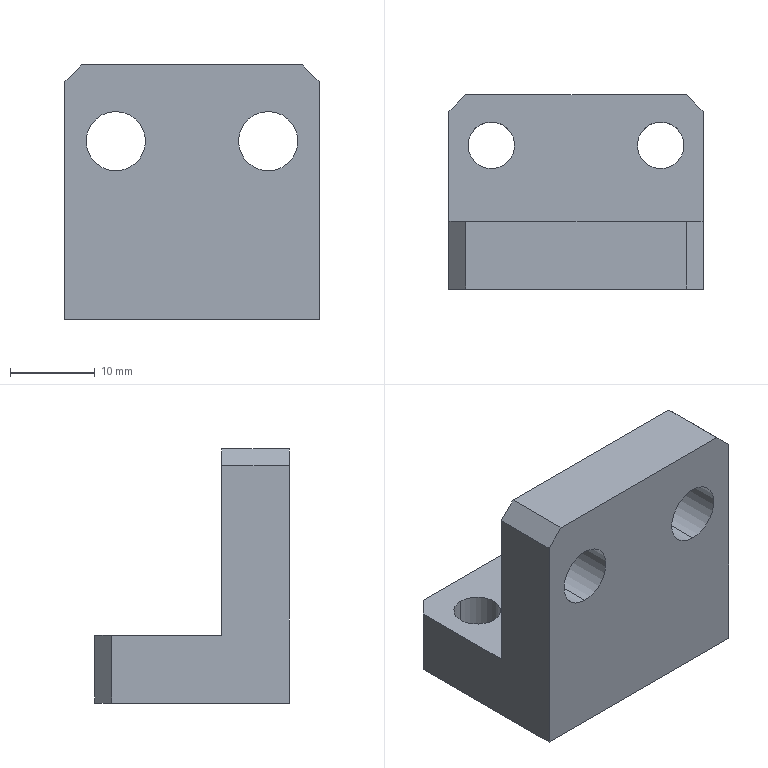Part | SolidWorks | features BaseBody 1 | 1 solid | 20 faces | box 30.001 x 23.001 x 30 mm | volume 9740 mm3 | plane 12 | cylinder 8 | commonest cylinder face diameters 5.5 x4 7 x4
STEP:
#1=CARTESIAN_POINT('',(-621.131,675.797,346.732));
#2=VERTEX_POINT('',#1);
#3=CARTESIAN_POINT('',(-619.131,675.797,344.732));
#4=VERTEX_POINT('',#3);
#5=CARTESIAN_POINT('',(-621.131,675.797,346.732));
#6=DIRECTION('',(0.7071,-0.00003242,-0.7071));
#7=VECTOR('',#6,1000.);
#8=LINE('',#5,#7);
#9=EDGE_CURVE('',#2,#4,#8,.T.);
#10=ORIENTED_EDGE('',*,*,#9,.T.);
#11=CARTESIAN_POINT('',(-619.131,683.797,344.732));
#12=VERTEX_POINT('',#11);
#13=CARTESIAN_POINT('',(-619.131,683.797,344.732));
#14=DIRECTION('',(-0.00004584,-1.,0.));
#15=VECTOR('',#14,1000.);
#16=LINE('',#13,#15);
#17=EDGE_CURVE('',#12,#4,#16,.T.);
#18=ORIENTED_EDGE('',*,*,#17,.F.);
#19=CARTESIAN_POINT('',(-621.131,683.797,346.732));
#20=VERTEX_POINT('',#19);
#21=CARTESIAN_POINT('',(-619.131,683.797,344.732));
#22=DIRECTION('',(-0.7071,0.00003242,0.7071));
#23=VECTOR('',#22,1000.);
#24=LINE('',#21,#23);
#25=EDGE_CURVE('',#12,#20,#24,.T.);
#26=ORIENTED_EDGE('',*,*,#25,.T.);
#27=CARTESIAN_POINT('',(-621.131,675.797,346.732));
#28=DIRECTION('',(0.00004584,1.,0.));
#29=VECTOR('',#28,1000.);
#30=LINE('',#27,#29);
#31=EDGE_CURVE('',#2,#20,#30,.T.);
#32=ORIENTED_EDGE('',*,*,#31,.F.);
#33=EDGE_LOOP('',(#10,#18,#26,#32));
#34=FACE_OUTER_BOUND('',#33,.T.);
#35=CARTESIAN_POINT('',(-619.131,675.797,344.732));
#36=DIRECTION('',(-0.7071,0.00003242,-0.7071));
#37=DIRECTION('',(0.00004584,1.,0.));
#38=AXIS2_PLACEMENT_3D('',#35,#36,#37);
#39=PLANE('',#38);
#40=ADVANCED_FACE('',(#34),#39,.F.);
#41=CARTESIAN_POINT('',(-647.131,675.798,346.732));
#42=VERTEX_POINT('',#41);
#43=CARTESIAN_POINT('',(-647.131,675.798,346.732));
#44=DIRECTION('',(1.,-0.00004584,0.));
#45=VECTOR('',#44,1000.);
#46=LINE('',#43,#45);
#47=EDGE_CURVE('',#42,#2,#46,.T.);
#48=ORIENTED_EDGE('',*,*,#47,.T.);
#49=ORIENTED_EDGE('',*,*,#31,.T.);
#50=CARTESIAN_POINT('',(-647.131,683.798,346.732));
#51=VERTEX_POINT('',#50);
#52=CARTESIAN_POINT('',(-621.131,683.797,346.732));
#53=DIRECTION('',(-1.,0.00004584,0.));
#54=VECTOR('',#53,1000.);
#55=LINE('',#52,#54);
#56=EDGE_CURVE('',#20,#51,#55,.T.);
#57=ORIENTED_EDGE('',*,*,#56,.T.);
#58=CARTESIAN_POINT('',(-647.131,675.798,346.732));
#59=DIRECTION('',(0.00004584,1.,0.));
#60=VECTOR('',#59,1000.);
#61=LINE('',#58,#60);
#62=EDGE_CURVE('',#42,#51,#61,.T.);
#63=ORIENTED_EDGE('',*,*,#62,.F.);
#64=EDGE_LOOP('',(#48,#49,#57,#63));
#65=FACE_OUTER_BOUND('',#64,.T.);
#66=CARTESIAN_POINT('',(-619.131,675.797,346.732));
#67=DIRECTION('',(0.,0.,-1.));
#68=DIRECTION('',(-0.00004584,-1.,0.));
#69=AXIS2_PLACEMENT_3D('',#66,#67,#68);
#70=PLANE('',#69);
#71=ADVANCED_FACE('',(#65),#70,.F.);
#72=CARTESIAN_POINT('',(-649.131,675.798,344.732));
#73=VERTEX_POINT('',#72);
#74=CARTESIAN_POINT('',(-649.131,675.798,344.732));
#75=DIRECTION('',(0.7071,-0.00003242,0.7071));
#76=VECTOR('',#75,1000.);
#77=LINE('',#74,#76);
#78=EDGE_CURVE('',#73,#42,#77,.T.);
#79=ORIENTED_EDGE('',*,*,#78,.T.);
#80=ORIENTED_EDGE('',*,*,#62,.T.);
#81=CARTESIAN_POINT('',(-649.131,683.798,344.732));
#82=VERTEX_POINT('',#81);
#83=CARTESIAN_POINT('',(-647.131,683.798,346.732));
#84=DIRECTION('',(-0.7071,0.00003242,-0.7071));
#85=VECTOR('',#84,1000.);
#86=LINE('',#83,#85);
#87=EDGE_CURVE('',#51,#82,#86,.T.);
#88=ORIENTED_EDGE('',*,*,#87,.T.);
#89=CARTESIAN_POINT('',(-649.131,683.798,344.732));
#90=DIRECTION('',(-0.00004584,-1.,0.));
#91=VECTOR('',#90,1000.);
#92=LINE('',#89,#91);
#93=EDGE_CURVE('',#82,#73,#92,.T.);
#94=ORIENTED_EDGE('',*,*,#93,.T.);
#95=EDGE_LOOP('',(#79,#80,#88,#94));
#96=FACE_OUTER_BOUND('',#95,.T.);
#97=CARTESIAN_POINT('',(-647.131,675.798,346.732));
#98=DIRECTION('',(-0.7071,0.00003242,0.7071));
#99=DIRECTION('',(-0.00004584,-1.,0.));
#100=AXIS2_PLACEMENT_3D('',#97,#98,#99);
#101=PLANE('',#100);
#102=ADVANCED_FACE('',(#96),#101,.T.);
#103=CARTESIAN_POINT('',(-649.131,675.798,316.732));
#104=VERTEX_POINT('',#103);
#105=CARTESIAN_POINT('',(-649.13,696.798,316.732));
#106=VERTEX_POINT('',#105);
#107=CARTESIAN_POINT('',(-649.131,675.798,316.732));
#108=DIRECTION('',(0.00004584,1.,0.));
#109=VECTOR('',#108,1000.);
#110=LINE('',#107,#109);
#111=EDGE_CURVE('',#104,#106,#110,.T.);
#112=ORIENTED_EDGE('',*,*,#111,.F.);
#113=CARTESIAN_POINT('',(-649.131,675.798,344.732));
#114=DIRECTION('',(0.,0.,-1.));
#115=VECTOR('',#114,1000.);
#116=LINE('',#113,#115);
#117=EDGE_CURVE('',#73,#104,#116,.T.);
#118=ORIENTED_EDGE('',*,*,#117,.F.);
#119=ORIENTED_EDGE('',*,*,#93,.F.);
#120=CARTESIAN_POINT('',(-649.131,683.798,324.732));
#121=VERTEX_POINT('',#120);
#122=CARTESIAN_POINT('',(-649.131,683.798,344.732));
#123=DIRECTION('',(0.,0.,-1.));
#124=VECTOR('',#123,1000.);
#125=LINE('',#122,#124);
#126=EDGE_CURVE('',#82,#121,#125,.T.);
#127=ORIENTED_EDGE('',*,*,#126,.T.);
#128=CARTESIAN_POINT('',(-649.13,696.798,324.732));
#129=VERTEX_POINT('',#128);
#130=CARTESIAN_POINT('',(-649.13,696.798,324.732));
#131=DIRECTION('',(-0.00004584,-1.,0.));
#132=VECTOR('',#131,1000.);
#133=LINE('',#130,#132);
#134=EDGE_CURVE('',#129,#121,#133,.T.);
#135=ORIENTED_EDGE('',*,*,#134,.F.);
#136=CARTESIAN_POINT('',(-649.13,696.798,316.732));
#137=DIRECTION('',(0.,0.,1.));
#138=VECTOR('',#137,1000.);
#139=LINE('',#136,#138);
#140=EDGE_CURVE('',#106,#129,#139,.T.);
#141=ORIENTED_EDGE('',*,*,#140,.F.);
#142=EDGE_LOOP('',(#112,#118,#119,#127,#135,#141));
#143=FACE_OUTER_BOUND('',#142,.T.);
#144=CARTESIAN_POINT('',(-649.131,675.798,316.732));
#145=DIRECTION('',(-1.,0.00004584,0.));
#146=DIRECTION('',(0.,0.,-1.));
#147=AXIS2_PLACEMENT_3D('',#144,#145,#146);
#148=PLANE('',#147);
#149=ADVANCED_FACE('',(#143),#148,.T.);
#150=CARTESIAN_POINT('',(-647.13,698.798,324.732));
#151=VERTEX_POINT('',#150);
#152=CARTESIAN_POINT('',(-649.13,696.798,324.732));
#153=DIRECTION('',(0.7071,0.7071,0.));
#154=VECTOR('',#153,1000.);
#155=LINE('',#152,#154);
#156=EDGE_CURVE('',#129,#151,#155,.T.);
#157=ORIENTED_EDGE('',*,*,#156,.T.);
#158=CARTESIAN_POINT('',(-647.13,698.798,316.732));
#159=VERTEX_POINT('',#158);
#160=CARTESIAN_POINT('',(-647.13,698.798,324.732));
#161=DIRECTION('',(0.,0.,-1.));
#162=VECTOR('',#161,1000.);
#163=LINE('',#160,#162);
#164=EDGE_CURVE('',#151,#159,#163,.T.);
#165=ORIENTED_EDGE('',*,*,#164,.T.);
#166=CARTESIAN_POINT('',(-647.13,698.798,316.732));
#167=DIRECTION('',(-0.7071,-0.7071,0.));
#168=VECTOR('',#167,1000.);
#169=LINE('',#166,#168);
#170=EDGE_CURVE('',#159,#106,#169,.T.);
#171=ORIENTED_EDGE('',*,*,#170,.T.);
#172=ORIENTED_EDGE('',*,*,#140,.T.);
#173=EDGE_LOOP('',(#157,#165,#171,#172));
#174=FACE_OUTER_BOUND('',#173,.T.);
#175=CARTESIAN_POINT('',(-647.13,698.798,324.732));
#176=DIRECTION('',(-0.7071,0.7071,0.));
#177=DIRECTION('',(-0.7071,-0.7071,0.));
#178=AXIS2_PLACEMENT_3D('',#175,#176,#177);
#179=PLANE('',#178);
#180=ADVANCED_FACE('',(#174),#179,.T.);
#181=CARTESIAN_POINT('',(-621.13,698.797,316.732));
#182=VERTEX_POINT('',#181);
#183=CARTESIAN_POINT('',(-647.13,698.798,316.732));
#184=DIRECTION('',(1.,-0.00004584,0.));
#185=VECTOR('',#184,1000.);
#186=LINE('',#183,#185);
#187=EDGE_CURVE('',#159,#182,#186,.T.);
#188=ORIENTED_EDGE('',*,*,#187,.T.);
#189=CARTESIAN_POINT('',(-619.13,696.797,316.732));
#190=VERTEX_POINT('',#189);
#191=CARTESIAN_POINT('',(-619.13,696.797,316.732));
#192=DIRECTION('',(-0.7071,0.7071,0.));
#193=VECTOR('',#192,1000.);
#194=LINE('',#191,#193);
#195=EDGE_CURVE('',#190,#182,#194,.T.);
#196=ORIENTED_EDGE('',*,*,#195,.F.);
#197=CARTESIAN_POINT('',(-619.131,675.797,316.732));
#198=VERTEX_POINT('',#197);
#199=CARTESIAN_POINT('',(-619.131,675.797,316.732));
#200=DIRECTION('',(0.00004584,1.,0.));
#201=VECTOR('',#200,1000.);
#202=LINE('',#199,#201);
#203=EDGE_CURVE('',#198,#190,#202,.T.);
#204=ORIENTED_EDGE('',*,*,#203,.F.);
#205=CARTESIAN_POINT('',(-649.131,675.798,316.732));
#206=DIRECTION('',(1.,-0.00004584,0.));
#207=VECTOR('',#206,1000.);
#208=LINE('',#205,#207);
#209=EDGE_CURVE('',#104,#198,#208,.T.);
#210=ORIENTED_EDGE('',*,*,#209,.F.);
#211=ORIENTED_EDGE('',*,*,#111,.T.);
#212=ORIENTED_EDGE('',*,*,#170,.F.);
#213=EDGE_LOOP('',(#188,#196,#204,#210,#211,#212));
#214=FACE_OUTER_BOUND('',#213,.T.);
#215=CARTESIAN_POINT('',(-624.131,695.547,316.732));
#216=VERTEX_POINT('',#215);
#217=CARTESIAN_POINT('',(-624.131,690.047,316.732));
#218=VERTEX_POINT('',#217);
#219=CARTESIAN_POINT('',(-624.131,692.797,316.732));
#220=DIRECTION('',(0.,0.,-1.));
#221=DIRECTION('',(0.00004584,1.,0.));
#222=AXIS2_PLACEMENT_3D('',#219,#220,#221);
#223=CIRCLE('',#222,2.75);
#224=EDGE_CURVE('',#216,#218,#223,.T.);
#225=ORIENTED_EDGE('',*,*,#224,.F.);
#226=CARTESIAN_POINT('',(-624.131,692.797,316.732));
#227=DIRECTION('',(0.,0.,-1.));
#228=DIRECTION('',(-0.00004584,-1.,0.));
#229=AXIS2_PLACEMENT_3D('',#226,#227,#228);
#230=CIRCLE('',#229,2.75);
#231=EDGE_CURVE('',#218,#216,#230,.T.);
#232=ORIENTED_EDGE('',*,*,#231,.F.);
#233=EDGE_LOOP('',(#225,#232));
#234=FACE_BOUND('',#233,.T.);
#235=CARTESIAN_POINT('',(-644.131,695.548,316.732));
#236=VERTEX_POINT('',#235);
#237=CARTESIAN_POINT('',(-644.131,690.048,316.732));
#238=VERTEX_POINT('',#237);
#239=CARTESIAN_POINT('',(-644.131,692.798,316.732));
#240=DIRECTION('',(0.,0.,-1.));
#241=DIRECTION('',(0.00004584,1.,0.));
#242=AXIS2_PLACEMENT_3D('',#239,#240,#241);
#243=CIRCLE('',#242,2.75);
#244=EDGE_CURVE('',#236,#238,#243,.T.);
#245=ORIENTED_EDGE('',*,*,#244,.F.);
#246=CARTESIAN_POINT('',(-644.131,692.798,316.732));
#247=DIRECTION('',(0.,0.,-1.));
#248=DIRECTION('',(-0.00004584,-1.,0.));
#249=AXIS2_PLACEMENT_3D('',#246,#247,#248);
#250=CIRCLE('',#249,2.75);
#251=EDGE_CURVE('',#238,#236,#250,.T.);
#252=ORIENTED_EDGE('',*,*,#251,.F.);
#253=EDGE_LOOP('',(#245,#252));
#254=FACE_BOUND('',#253,.T.);
#255=CARTESIAN_POINT('',(-619.131,675.797,316.732));
#256=DIRECTION('',(0.,0.,1.));
#257=DIRECTION('',(0.00004584,1.,0.));
#258=AXIS2_PLACEMENT_3D('',#255,#256,#257);
#259=PLANE('',#258);
#260=ADVANCED_FACE('',(#214,#234,#254),#259,.F.);
#261=ORIENTED_EDGE('',*,*,#117,.T.);
#262=ORIENTED_EDGE('',*,*,#209,.T.);
#263=CARTESIAN_POINT('',(-619.131,675.797,344.732));
#264=DIRECTION('',(0.,0.,-1.));
#265=VECTOR('',#264,1000.);
#266=LINE('',#263,#265);
#267=EDGE_CURVE('',#4,#198,#266,.T.);
#268=ORIENTED_EDGE('',*,*,#267,.F.);
#269=ORIENTED_EDGE('',*,*,#9,.F.);
#270=ORIENTED_EDGE('',*,*,#47,.F.);
#271=ORIENTED_EDGE('',*,*,#78,.F.);
#272=EDGE_LOOP('',(#261,#262,#268,#269,#270,#271));
#273=FACE_OUTER_BOUND('',#272,.T.);
#274=CARTESIAN_POINT('',(-625.131,675.797,334.232));
#275=VERTEX_POINT('',#274);
#276=CARTESIAN_POINT('',(-625.131,675.797,341.232));
#277=VERTEX_POINT('',#276);
#278=CARTESIAN_POINT('',(-625.131,675.797,337.732));
#279=DIRECTION('',(-0.00004584,-1.,0.));
#280=DIRECTION('',(0.,0.,-1.));
#281=AXIS2_PLACEMENT_3D('',#278,#279,#280);
#282=CIRCLE('',#281,3.5);
#283=EDGE_CURVE('',#275,#277,#282,.T.);
#284=ORIENTED_EDGE('',*,*,#283,.F.);
#285=CARTESIAN_POINT('',(-625.131,675.797,337.732));
#286=DIRECTION('',(-0.00004584,-1.,0.));
#287=DIRECTION('',(0.,0.,1.));
#288=AXIS2_PLACEMENT_3D('',#285,#286,#287);
#289=CIRCLE('',#288,3.5);
#290=EDGE_CURVE('',#277,#275,#289,.T.);
#291=ORIENTED_EDGE('',*,*,#290,.F.);
#292=EDGE_LOOP('',(#284,#291));
#293=FACE_BOUND('',#292,.T.);
#294=CARTESIAN_POINT('',(-643.131,675.798,334.232));
#295=VERTEX_POINT('',#294);
#296=CARTESIAN_POINT('',(-643.131,675.798,341.232));
#297=VERTEX_POINT('',#296);
#298=CARTESIAN_POINT('',(-643.131,675.798,337.732));
#299=DIRECTION('',(-0.00004584,-1.,0.));
#300=DIRECTION('',(0.,0.,-1.));
#301=AXIS2_PLACEMENT_3D('',#298,#299,#300);
#302=CIRCLE('',#301,3.5);
#303=EDGE_CURVE('',#295,#297,#302,.T.);
#304=ORIENTED_EDGE('',*,*,#303,.F.);
#305=CARTESIAN_POINT('',(-643.131,675.798,337.732));
#306=DIRECTION('',(-0.00004584,-1.,0.));
#307=DIRECTION('',(0.,0.,1.));
#308=AXIS2_PLACEMENT_3D('',#305,#306,#307);
#309=CIRCLE('',#308,3.5);
#310=EDGE_CURVE('',#297,#295,#309,.T.);
#311=ORIENTED_EDGE('',*,*,#310,.F.);
#312=EDGE_LOOP('',(#304,#311));
#313=FACE_BOUND('',#312,.T.);
#314=CARTESIAN_POINT('',(-619.131,675.797,316.732));
#315=DIRECTION('',(0.00004584,1.,0.));
#316=DIRECTION('',(0.,0.,-1.));
#317=AXIS2_PLACEMENT_3D('',#314,#315,#316);
#318=PLANE('',#317);
#319=ADVANCED_FACE('',(#273,#293,#313),#318,.F.);
#320=CARTESIAN_POINT('',(-619.13,696.797,324.732));
#321=VERTEX_POINT('',#320);
#322=CARTESIAN_POINT('',(-619.131,683.797,324.732));
#323=VERTEX_POINT('',#322);
#324=CARTESIAN_POINT('',(-619.13,696.797,324.732));
#325=DIRECTION('',(-0.00004584,-1.,0.));
#326=VECTOR('',#325,1000.);
#327=LINE('',#324,#326);
#328=EDGE_CURVE('',#321,#323,#327,.T.);
#329=ORIENTED_EDGE('',*,*,#328,.T.);
#330=CARTESIAN_POINT('',(-619.131,683.797,324.732));
#331=DIRECTION('',(0.,0.,1.));
#332=VECTOR('',#331,1000.);
#333=LINE('',#330,#332);
#334=EDGE_CURVE('',#323,#12,#333,.T.);
#335=ORIENTED_EDGE('',*,*,#334,.T.);
#336=ORIENTED_EDGE('',*,*,#17,.T.);
#337=ORIENTED_EDGE('',*,*,#267,.T.);
#338=ORIENTED_EDGE('',*,*,#203,.T.);
#339=CARTESIAN_POINT('',(-619.13,696.797,324.732));
#340=DIRECTION('',(0.,0.,-1.));
#341=VECTOR('',#340,1000.);
#342=LINE('',#339,#341);
#343=EDGE_CURVE('',#321,#190,#342,.T.);
#344=ORIENTED_EDGE('',*,*,#343,.F.);
#345=EDGE_LOOP('',(#329,#335,#336,#337,#338,#344));
#346=FACE_OUTER_BOUND('',#345,.T.);
#347=CARTESIAN_POINT('',(-619.131,675.797,316.732));
#348=DIRECTION('',(-1.,0.00004584,0.));
#349=DIRECTION('',(0.,0.,-1.));
#350=AXIS2_PLACEMENT_3D('',#347,#348,#349);
#351=PLANE('',#350);
#352=ADVANCED_FACE('',(#346),#351,.F.);
#353=CARTESIAN_POINT('',(-621.13,698.797,324.732));
#354=VERTEX_POINT('',#353);
#355=CARTESIAN_POINT('',(-621.13,698.797,324.732));
#356=DIRECTION('',(0.7071,-0.7071,0.));
#357=VECTOR('',#356,1000.);
#358=LINE('',#355,#357);
#359=EDGE_CURVE('',#354,#321,#358,.T.);
#360=ORIENTED_EDGE('',*,*,#359,.T.);
#361=ORIENTED_EDGE('',*,*,#343,.T.);
#362=ORIENTED_EDGE('',*,*,#195,.T.);
#363=CARTESIAN_POINT('',(-621.13,698.797,316.732));
#364=DIRECTION('',(0.,0.,1.));
#365=VECTOR('',#364,1000.);
#366=LINE('',#363,#365);
#367=EDGE_CURVE('',#182,#354,#366,.T.);
#368=ORIENTED_EDGE('',*,*,#367,.T.);
#369=EDGE_LOOP('',(#360,#361,#362,#368));
#370=FACE_OUTER_BOUND('',#369,.T.);
#371=CARTESIAN_POINT('',(-619.13,696.797,316.732));
#372=DIRECTION('',(-0.7071,-0.7071,0.));
#373=DIRECTION('',(0.,0.,-1.));
#374=AXIS2_PLACEMENT_3D('',#371,#372,#373);
#375=PLANE('',#374);
#376=ADVANCED_FACE('',(#370),#375,.F.);
#377=CARTESIAN_POINT('',(-647.13,698.798,324.732));
#378=DIRECTION('',(1.,-0.00004584,0.));
#379=VECTOR('',#378,1000.);
#380=LINE('',#377,#379);
#381=EDGE_CURVE('',#151,#354,#380,.T.);
#382=ORIENTED_EDGE('',*,*,#381,.T.);
#383=ORIENTED_EDGE('',*,*,#367,.F.);
#384=ORIENTED_EDGE('',*,*,#187,.F.);
#385=ORIENTED_EDGE('',*,*,#164,.F.);
#386=EDGE_LOOP('',(#382,#383,#384,#385));
#387=FACE_OUTER_BOUND('',#386,.T.);
#388=CARTESIAN_POINT('',(-619.13,698.797,324.732));
#389=DIRECTION('',(-0.00004584,-1.,0.));
#390=DIRECTION('',(0.,0.,1.));
#391=AXIS2_PLACEMENT_3D('',#388,#389,#390);
#392=PLANE('',#391);
#393=ADVANCED_FACE('',(#387),#392,.F.);
#394=ORIENTED_EDGE('',*,*,#134,.T.);
#395=CARTESIAN_POINT('',(-649.131,683.798,324.732));
#396=DIRECTION('',(1.,-0.00004584,0.));
#397=VECTOR('',#396,1000.);
#398=LINE('',#395,#397);
#399=EDGE_CURVE('',#121,#323,#398,.T.);
#400=ORIENTED_EDGE('',*,*,#399,.T.);
#401=ORIENTED_EDGE('',*,*,#328,.F.);
#402=ORIENTED_EDGE('',*,*,#359,.F.);
#403=ORIENTED_EDGE('',*,*,#381,.F.);
#404=ORIENTED_EDGE('',*,*,#156,.F.);
#405=EDGE_LOOP('',(#394,#400,#401,#402,#403,#404));
#406=FACE_OUTER_BOUND('',#405,.T.);
#407=CARTESIAN_POINT('',(-624.131,690.047,324.732));
#408=VERTEX_POINT('',#407);
#409=CARTESIAN_POINT('',(-624.131,695.547,324.732));
#410=VERTEX_POINT('',#409);
#411=CARTESIAN_POINT('',(-624.131,692.797,324.732));
#412=DIRECTION('',(0.,0.,1.));
#413=DIRECTION('',(-0.00004584,-1.,0.));
#414=AXIS2_PLACEMENT_3D('',#411,#412,#413);
#415=CIRCLE('',#414,2.75);
#416=EDGE_CURVE('',#408,#410,#415,.T.);
#417=ORIENTED_EDGE('',*,*,#416,.F.);
#418=CARTESIAN_POINT('',(-624.131,692.797,324.732));
#419=DIRECTION('',(0.,0.,1.));
#420=DIRECTION('',(0.00004584,1.,0.));
#421=AXIS2_PLACEMENT_3D('',#418,#419,#420);
#422=CIRCLE('',#421,2.75);
#423=EDGE_CURVE('',#410,#408,#422,.T.);
#424=ORIENTED_EDGE('',*,*,#423,.F.);
#425=EDGE_LOOP('',(#417,#424));
#426=FACE_BOUND('',#425,.T.);
#427=CARTESIAN_POINT('',(-644.131,690.048,324.732));
#428=VERTEX_POINT('',#427);
#429=CARTESIAN_POINT('',(-644.131,695.548,324.732));
#430=VERTEX_POINT('',#429);
#431=CARTESIAN_POINT('',(-644.131,692.798,324.732));
#432=DIRECTION('',(0.,0.,1.));
#433=DIRECTION('',(-0.00004584,-1.,0.));
#434=AXIS2_PLACEMENT_3D('',#431,#432,#433);
#435=CIRCLE('',#434,2.75);
#436=EDGE_CURVE('',#428,#430,#435,.T.);
#437=ORIENTED_EDGE('',*,*,#436,.F.);
#438=CARTESIAN_POINT('',(-644.131,692.798,324.732));
#439=DIRECTION('',(0.,0.,1.));
#440=DIRECTION('',(0.00004584,1.,0.));
#441=AXIS2_PLACEMENT_3D('',#438,#439,#440);
#442=CIRCLE('',#441,2.75);
#443=EDGE_CURVE('',#430,#428,#442,.T.);
#444=ORIENTED_EDGE('',*,*,#443,.F.);
#445=EDGE_LOOP('',(#437,#444));
#446=FACE_BOUND('',#445,.T.);
#447=CARTESIAN_POINT('',(-619.131,683.797,324.732));
#448=DIRECTION('',(0.,0.,-1.));
#449=DIRECTION('',(-0.00004584,-1.,0.));
#450=AXIS2_PLACEMENT_3D('',#447,#448,#449);
#451=PLANE('',#450);
#452=ADVANCED_FACE('',(#406,#426,#446),#451,.F.);
#453=ORIENTED_EDGE('',*,*,#56,.F.);
#454=ORIENTED_EDGE('',*,*,#25,.F.);
#455=ORIENTED_EDGE('',*,*,#334,.F.);
#456=ORIENTED_EDGE('',*,*,#399,.F.);
#457=ORIENTED_EDGE('',*,*,#126,.F.);
#458=ORIENTED_EDGE('',*,*,#87,.F.);
#459=EDGE_LOOP('',(#453,#454,#455,#456,#457,#458));
#460=FACE_OUTER_BOUND('',#459,.T.);
#461=CARTESIAN_POINT('',(-625.131,683.797,341.232));
#462=VERTEX_POINT('',#461);
#463=CARTESIAN_POINT('',(-625.131,683.797,334.232));
#464=VERTEX_POINT('',#463);
#465=CARTESIAN_POINT('',(-625.131,683.797,337.732));
#466=DIRECTION('',(0.00004584,1.,0.));
#467=DIRECTION('',(0.,0.,1.));
#468=AXIS2_PLACEMENT_3D('',#465,#466,#467);
#469=CIRCLE('',#468,3.5);
#470=EDGE_CURVE('',#462,#464,#469,.T.);
#471=ORIENTED_EDGE('',*,*,#470,.F.);
#472=CARTESIAN_POINT('',(-625.131,683.797,337.732));
#473=DIRECTION('',(0.00004584,1.,0.));
#474=DIRECTION('',(0.,0.,-1.));
#475=AXIS2_PLACEMENT_3D('',#472,#473,#474);
#476=CIRCLE('',#475,3.5);
#477=EDGE_CURVE('',#464,#462,#476,.T.);
#478=ORIENTED_EDGE('',*,*,#477,.F.);
#479=EDGE_LOOP('',(#471,#478));
#480=FACE_BOUND('',#479,.T.);
#481=CARTESIAN_POINT('',(-643.131,683.798,341.232));
#482=VERTEX_POINT('',#481);
#483=CARTESIAN_POINT('',(-643.131,683.798,334.232));
#484=VERTEX_POINT('',#483);
#485=CARTESIAN_POINT('',(-643.131,683.798,337.732));
#486=DIRECTION('',(0.00004584,1.,0.));
#487=DIRECTION('',(0.,0.,1.));
#488=AXIS2_PLACEMENT_3D('',#485,#486,#487);
#489=CIRCLE('',#488,3.5);
#490=EDGE_CURVE('',#482,#484,#489,.T.);
#491=ORIENTED_EDGE('',*,*,#490,.F.);
#492=CARTESIAN_POINT('',(-643.131,683.798,337.732));
#493=DIRECTION('',(0.00004584,1.,0.));
#494=DIRECTION('',(0.,0.,-1.));
#495=AXIS2_PLACEMENT_3D('',#492,#493,#494);
#496=CIRCLE('',#495,3.5);
#497=EDGE_CURVE('',#484,#482,#496,.T.);
#498=ORIENTED_EDGE('',*,*,#497,.F.);
#499=EDGE_LOOP('',(#491,#498));
#500=FACE_BOUND('',#499,.T.);
#501=CARTESIAN_POINT('',(-619.131,683.797,346.732));
#502=DIRECTION('',(-0.00004584,-1.,0.));
#503=DIRECTION('',(0.,0.,1.));
#504=AXIS2_PLACEMENT_3D('',#501,#502,#503);
#505=PLANE('',#504);
#506=ADVANCED_FACE('',(#460,#480,#500),#505,.F.);
#507=ORIENTED_EDGE('',*,*,#477,.T.);
#508=CARTESIAN_POINT('',(-625.131,683.797,341.232));
#509=DIRECTION('',(-0.00004584,-1.,0.));
#510=VECTOR('',#509,1000.);
#511=LINE('',#508,#510);
#512=EDGE_CURVE('',#462,#277,#511,.T.);
#513=ORIENTED_EDGE('',*,*,#512,.T.);
#514=ORIENTED_EDGE('',*,*,#290,.T.);
#515=CARTESIAN_POINT('',(-625.131,675.797,334.232));
#516=DIRECTION('',(0.00004584,1.,0.));
#517=VECTOR('',#516,1000.);
#518=LINE('',#515,#517);
#519=EDGE_CURVE('',#275,#464,#518,.T.);
#520=ORIENTED_EDGE('',*,*,#519,.T.);
#521=EDGE_LOOP('',(#507,#513,#514,#520));
#522=FACE_OUTER_BOUND('',#521,.T.);
#523=CARTESIAN_POINT('',(-625.131,683.797,337.732));
#524=DIRECTION('',(0.00004584,1.,0.));
#525=DIRECTION('',(0.,0.,-1.));
#526=AXIS2_PLACEMENT_3D('',#523,#524,#525);
#527=CYLINDRICAL_SURFACE('',#526,3.5);
#528=ADVANCED_FACE('',(#522),#527,.F.);
#529=ORIENTED_EDGE('',*,*,#512,.F.);
#530=ORIENTED_EDGE('',*,*,#470,.T.);
#531=ORIENTED_EDGE('',*,*,#519,.F.);
#532=ORIENTED_EDGE('',*,*,#283,.T.);
#533=EDGE_LOOP('',(#529,#530,#531,#532));
#534=FACE_OUTER_BOUND('',#533,.T.);
#535=CARTESIAN_POINT('',(-625.131,683.797,337.732));
#536=DIRECTION('',(0.00004584,1.,0.));
#537=DIRECTION('',(0.,0.,-1.));
#538=AXIS2_PLACEMENT_3D('',#535,#536,#537);
#539=CYLINDRICAL_SURFACE('',#538,3.5);
#540=ADVANCED_FACE('',(#534),#539,.F.);
#541=ORIENTED_EDGE('',*,*,#497,.T.);
#542=CARTESIAN_POINT('',(-643.131,683.798,341.232));
#543=DIRECTION('',(-0.00004584,-1.,0.));
#544=VECTOR('',#543,1000.);
#545=LINE('',#542,#544);
#546=EDGE_CURVE('',#482,#297,#545,.T.);
#547=ORIENTED_EDGE('',*,*,#546,.T.);
#548=ORIENTED_EDGE('',*,*,#310,.T.);
#549=CARTESIAN_POINT('',(-643.131,675.798,334.232));
#550=DIRECTION('',(0.00004584,1.,0.));
#551=VECTOR('',#550,1000.);
#552=LINE('',#549,#551);
#553=EDGE_CURVE('',#295,#484,#552,.T.);
#554=ORIENTED_EDGE('',*,*,#553,.T.);
#555=EDGE_LOOP('',(#541,#547,#548,#554));
#556=FACE_OUTER_BOUND('',#555,.T.);
#557=CARTESIAN_POINT('',(-643.131,683.798,337.732));
#558=DIRECTION('',(0.00004584,1.,0.));
#559=DIRECTION('',(0.,0.,-1.));
#560=AXIS2_PLACEMENT_3D('',#557,#558,#559);
#561=CYLINDRICAL_SURFACE('',#560,3.5);
#562=ADVANCED_FACE('',(#556),#561,.F.);
#563=ORIENTED_EDGE('',*,*,#546,.F.);
#564=ORIENTED_EDGE('',*,*,#490,.T.);
#565=ORIENTED_EDGE('',*,*,#553,.F.);
#566=ORIENTED_EDGE('',*,*,#303,.T.);
#567=EDGE_LOOP('',(#563,#564,#565,#566));
#568=FACE_OUTER_BOUND('',#567,.T.);
#569=CARTESIAN_POINT('',(-643.131,683.798,337.732));
#570=DIRECTION('',(0.00004584,1.,0.));
#571=DIRECTION('',(0.,0.,-1.));
#572=AXIS2_PLACEMENT_3D('',#569,#570,#571);
#573=CYLINDRICAL_SURFACE('',#572,3.5);
#574=ADVANCED_FACE('',(#568),#573,.F.);
#575=ORIENTED_EDGE('',*,*,#423,.T.);
#576=CARTESIAN_POINT('',(-624.131,690.047,324.732));
#577=DIRECTION('',(0.,0.,-1.));
#578=VECTOR('',#577,1000.);
#579=LINE('',#576,#578);
#580=EDGE_CURVE('',#408,#218,#579,.T.);
#581=ORIENTED_EDGE('',*,*,#580,.T.);
#582=ORIENTED_EDGE('',*,*,#231,.T.);
#583=CARTESIAN_POINT('',(-624.131,695.547,316.732));
#584=DIRECTION('',(0.,0.,1.));
#585=VECTOR('',#584,1000.);
#586=LINE('',#583,#585);
#587=EDGE_CURVE('',#216,#410,#586,.T.);
#588=ORIENTED_EDGE('',*,*,#587,.T.);
#589=EDGE_LOOP('',(#575,#581,#582,#588));
#590=FACE_OUTER_BOUND('',#589,.T.);
#591=CARTESIAN_POINT('',(-624.131,692.797,324.732));
#592=DIRECTION('',(0.,0.,1.));
#593=DIRECTION('',(0.00004584,1.,0.));
#594=AXIS2_PLACEMENT_3D('',#591,#592,#593);
#595=CYLINDRICAL_SURFACE('',#594,2.75);
#596=ADVANCED_FACE('',(#590),#595,.F.);
#597=ORIENTED_EDGE('',*,*,#580,.F.);
#598=ORIENTED_EDGE('',*,*,#416,.T.);
#599=ORIENTED_EDGE('',*,*,#587,.F.);
#600=ORIENTED_EDGE('',*,*,#224,.T.);
#601=EDGE_LOOP('',(#597,#598,#599,#600));
#602=FACE_OUTER_BOUND('',#601,.T.);
#603=CARTESIAN_POINT('',(-624.131,692.797,324.732));
#604=DIRECTION('',(0.,0.,1.));
#605=DIRECTION('',(0.00004584,1.,0.));
#606=AXIS2_PLACEMENT_3D('',#603,#604,#605);
#607=CYLINDRICAL_SURFACE('',#606,2.75);
#608=ADVANCED_FACE('',(#602),#607,.F.);
#609=ORIENTED_EDGE('',*,*,#443,.T.);
#610=CARTESIAN_POINT('',(-644.131,690.048,324.732));
#611=DIRECTION('',(0.,0.,-1.));
#612=VECTOR('',#611,1000.);
#613=LINE('',#610,#612);
#614=EDGE_CURVE('',#428,#238,#613,.T.);
#615=ORIENTED_EDGE('',*,*,#614,.T.);
#616=ORIENTED_EDGE('',*,*,#251,.T.);
#617=CARTESIAN_POINT('',(-644.131,695.548,316.732));
#618=DIRECTION('',(0.,0.,1.));
#619=VECTOR('',#618,1000.);
#620=LINE('',#617,#619);
#621=EDGE_CURVE('',#236,#430,#620,.T.);
#622=ORIENTED_EDGE('',*,*,#621,.T.);
#623=EDGE_LOOP('',(#609,#615,#616,#622));
#624=FACE_OUTER_BOUND('',#623,.T.);
#625=CARTESIAN_POINT('',(-644.131,692.798,324.732));
#626=DIRECTION('',(0.,0.,1.));
#627=DIRECTION('',(0.00004584,1.,0.));
#628=AXIS2_PLACEMENT_3D('',#625,#626,#627);
#629=CYLINDRICAL_SURFACE('',#628,2.75);
#630=ADVANCED_FACE('',(#624),#629,.F.);
#631=ORIENTED_EDGE('',*,*,#614,.F.);
#632=ORIENTED_EDGE('',*,*,#436,.T.);
#633=ORIENTED_EDGE('',*,*,#621,.F.);
#634=ORIENTED_EDGE('',*,*,#244,.T.);
#635=EDGE_LOOP('',(#631,#632,#633,#634));
#636=FACE_OUTER_BOUND('',#635,.T.);
#637=CARTESIAN_POINT('',(-644.131,692.798,324.732));
#638=DIRECTION('',(0.,0.,1.));
#639=DIRECTION('',(0.00004584,1.,0.));
#640=AXIS2_PLACEMENT_3D('',#637,#638,#639);
#641=CYLINDRICAL_SURFACE('',#640,2.75);
#642=ADVANCED_FACE('',(#636),#641,.F.);
#643=CLOSED_SHELL('',(#40,#71,#102,#149,#180,#260,#319,#352,#376,#393,#452,#506,#528,#540,#562,#574,#596,#608,#630,#642));
#644=MANIFOLD_SOLID_BREP('',#643);
#645=CARTESIAN_POINT('',(0.,0.,0.));
#646=DIRECTION('',(0.,0.,1.));
#647=DIRECTION('',(1.,0.,0.));
#648=AXIS2_PLACEMENT_3D('',#645,#646,#647);
#649=(LENGTH_UNIT()NAMED_UNIT(*)SI_UNIT(.MILLI.,.METRE.));
#650=UNCERTAINTY_MEASURE_WITH_UNIT(LENGTH_MEASURE(0.00001),#649,'','');
#651=(NAMED_UNIT(*)PLANE_ANGLE_UNIT()SI_UNIT($,.RADIAN.));
#652=(NAMED_UNIT(*)SI_UNIT($,.STERADIAN.)SOLID_ANGLE_UNIT());
#653=(GEOMETRIC_REPRESENTATION_CONTEXT(3)GLOBAL_UNCERTAINTY_ASSIGNED_CONTEXT((#650))GLOBAL_UNIT_ASSIGNED_CONTEXT((#649,#651,#652))REPRESENTATION_CONTEXT('',''));
#654=ADVANCED_BREP_SHAPE_REPRESENTATION('',(#644,#648),#653);